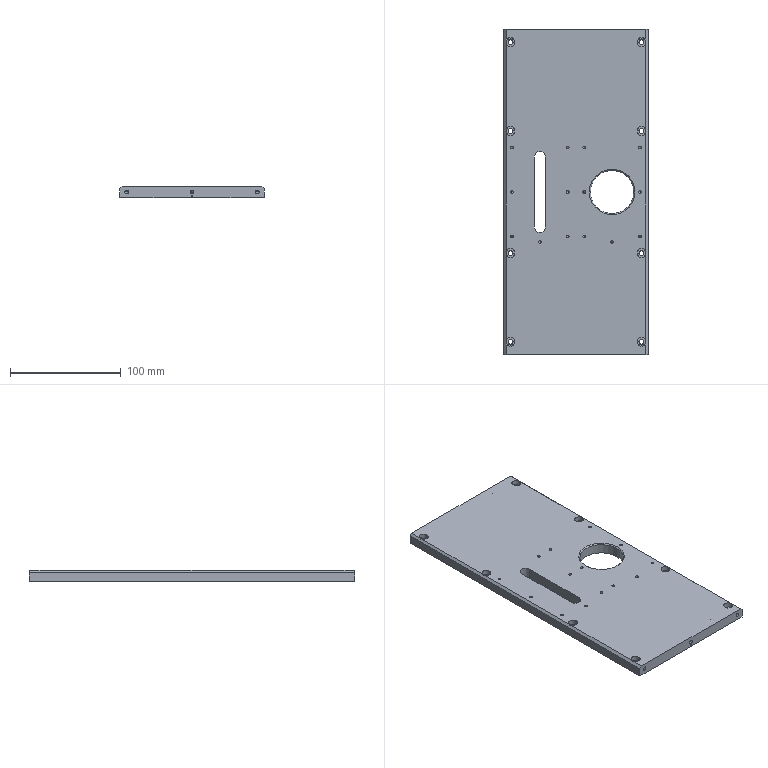Part | SolidWorks | features HoleWzd 5, MirrorPattern 4, Chamfer 2, Cut 2, Extrusion 1, ICE 1 | 1 solid | 140 faces | box 130 x 293 x 10 mm | volume 356054 mm3 | cylinder 80 | cone 38 | plane 22 | commonest cylinder face diameters 2.5 x32 4.5 x16 8 x16 3.3 x12 10 x2 39 x2